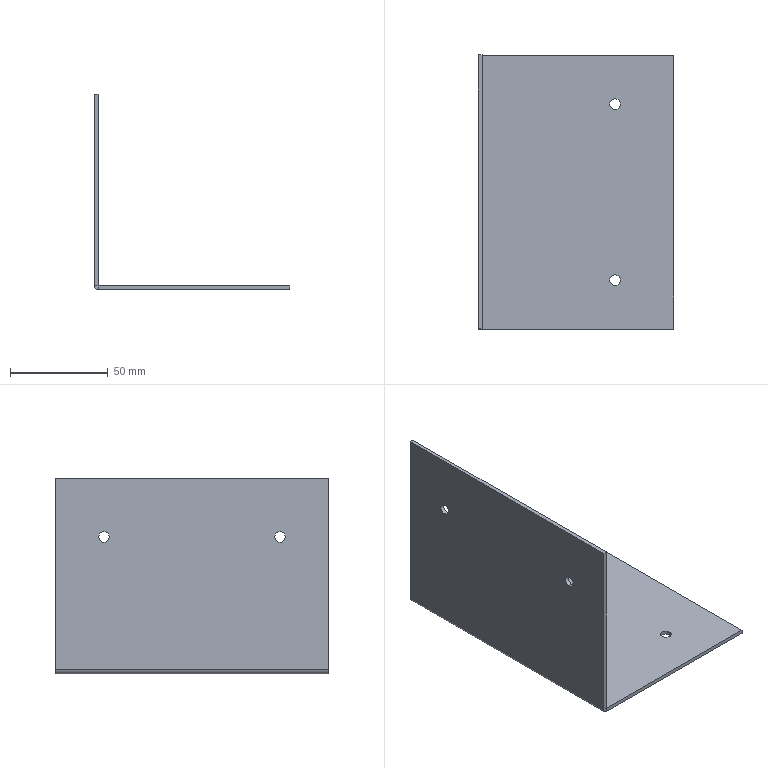Part | STEP file | Assembly TS-S07 | 1 solid | 22 faces | box 100 x 140 x 100 mm | volume 55113 mm3 | plane 12 | cylinder 10 | commonest cylinder face diameters 5.4 x8 0.4 x1 4.4 x1